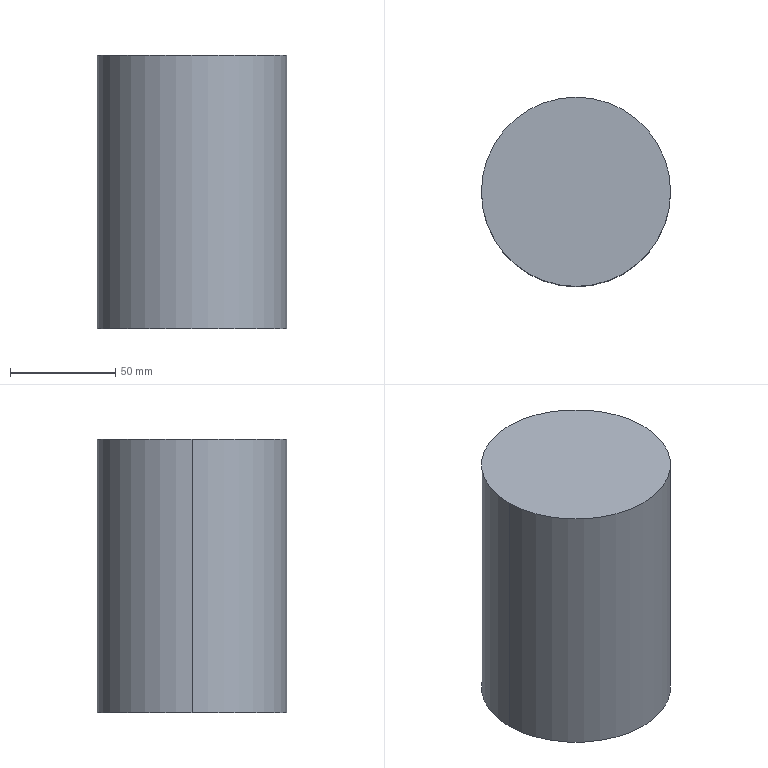Part | Creo | 1 solid | 11 faces | box 90 x 90 x 130 mm | volume 824415 mm3 | cylinder 6 | plane 3 | cone 2 | commonest cylinder face diameters 10.5 x2 12 x2 90 x2
STEP:
#1=CARTESIAN_POINT('',(-40.,-90.005,-201.));
#2=VERTEX_POINT('',#1);
#3=CARTESIAN_POINT('',(50.,-90.005,-201.));
#4=VERTEX_POINT('',#3);
#5=CARTESIAN_POINT('',(5.,-90.005,-201.));
#6=DIRECTION('',(0.,0.,1.));
#7=DIRECTION('',(-1.,0.,0.));
#8=AXIS2_PLACEMENT_3D('',#5,#6,#7);
#9=CIRCLE('',#8,45.);
#10=EDGE_CURVE('',#2,#4,#9,.T.);
#11=ORIENTED_EDGE('',*,*,#10,.F.);
#12=CARTESIAN_POINT('',(5.,-90.005,-201.));
#13=DIRECTION('',(0.,0.,1.));
#14=DIRECTION('',(1.,0.,0.));
#15=AXIS2_PLACEMENT_3D('',#12,#13,#14);
#16=CIRCLE('',#15,45.);
#17=EDGE_CURVE('',#4,#2,#16,.T.);
#18=ORIENTED_EDGE('',*,*,#17,.F.);
#19=EDGE_LOOP('',(#11,#18));
#20=FACE_OUTER_BOUND('',#19,.F.);
#21=CARTESIAN_POINT('',(5.,-58.005,-201.));
#22=DIRECTION('',(0.,0.,-1.));
#23=DIRECTION('',(0.,1.,0.));
#24=AXIS2_PLACEMENT_3D('',#21,#22,#23);
#25=PLANE('',#24);
#26=ADVANCED_FACE('',(#20),#25,.F.);
#27=ORIENTED_EDGE('',*,*,#10,.T.);
#28=CARTESIAN_POINT('',(50.,-90.005,-331.));
#29=VERTEX_POINT('',#28);
#30=CARTESIAN_POINT('',(50.,-90.005,-331.));
#31=DIRECTION('',(0.,0.,1.));
#32=VECTOR('',#31,130.);
#33=LINE('',#30,#32);
#34=EDGE_CURVE('',#29,#4,#33,.T.);
#35=ORIENTED_EDGE('',*,*,#34,.F.);
#36=CARTESIAN_POINT('',(-40.,-90.005,-331.));
#37=VERTEX_POINT('',#36);
#38=CARTESIAN_POINT('',(5.,-90.005,-331.));
#39=DIRECTION('',(0.,0.,-1.));
#40=DIRECTION('',(1.,0.,0.));
#41=AXIS2_PLACEMENT_3D('',#38,#39,#40);
#42=CIRCLE('',#41,45.);
#43=EDGE_CURVE('',#29,#37,#42,.T.);
#44=ORIENTED_EDGE('',*,*,#43,.T.);
#45=CARTESIAN_POINT('',(-40.,-90.005,-331.));
#46=DIRECTION('',(0.,0.,1.));
#47=VECTOR('',#46,130.);
#48=LINE('',#45,#47);
#49=EDGE_CURVE('',#37,#2,#48,.T.);
#50=ORIENTED_EDGE('',*,*,#49,.T.);
#51=EDGE_LOOP('',(#27,#35,#44,#50));
#52=FACE_OUTER_BOUND('',#51,.F.);
#53=CARTESIAN_POINT('',(5.,-90.005,-401.));
#54=DIRECTION('',(0.,0.,1.));
#55=DIRECTION('',(1.,0.,0.));
#56=AXIS2_PLACEMENT_3D('',#53,#54,#55);
#57=CYLINDRICAL_SURFACE('',#56,45.);
#58=ADVANCED_FACE('',(#52),#57,.T.);
#59=ORIENTED_EDGE('',*,*,#17,.T.);
#60=ORIENTED_EDGE('',*,*,#49,.F.);
#61=CARTESIAN_POINT('',(5.,-90.005,-331.));
#62=DIRECTION('',(0.,0.,-1.));
#63=DIRECTION('',(-1.,0.,0.));
#64=AXIS2_PLACEMENT_3D('',#61,#62,#63);
#65=CIRCLE('',#64,45.);
#66=EDGE_CURVE('',#37,#29,#65,.T.);
#67=ORIENTED_EDGE('',*,*,#66,.T.);
#68=ORIENTED_EDGE('',*,*,#34,.T.);
#69=EDGE_LOOP('',(#59,#60,#67,#68));
#70=FACE_OUTER_BOUND('',#69,.F.);
#71=CARTESIAN_POINT('',(5.,-90.005,-401.));
#72=DIRECTION('',(0.,0.,1.));
#73=DIRECTION('',(1.,0.,0.));
#74=AXIS2_PLACEMENT_3D('',#71,#72,#73);
#75=CYLINDRICAL_SURFACE('',#74,45.);
#76=ADVANCED_FACE('',(#70),#75,.T.);
#77=ORIENTED_EDGE('',*,*,#43,.F.);
#78=ORIENTED_EDGE('',*,*,#66,.F.);
#79=EDGE_LOOP('',(#77,#78));
#80=FACE_OUTER_BOUND('',#79,.F.);
#81=CARTESIAN_POINT('',(11.,-90.005,-331.));
#82=VERTEX_POINT('',#81);
#83=CARTESIAN_POINT('',(-1.,-90.005,-331.));
#84=VERTEX_POINT('',#83);
#85=CARTESIAN_POINT('',(5.,-90.005,-331.));
#86=DIRECTION('',(0.,0.,1.));
#87=DIRECTION('',(1.,0.,0.));
#88=AXIS2_PLACEMENT_3D('',#85,#86,#87);
#89=CIRCLE('',#88,6.);
#90=EDGE_CURVE('',#82,#84,#89,.T.);
#91=ORIENTED_EDGE('',*,*,#90,.F.);
#92=CARTESIAN_POINT('',(5.,-90.005,-331.));
#93=DIRECTION('',(0.,0.,1.));
#94=DIRECTION('',(-1.,0.,0.));
#95=AXIS2_PLACEMENT_3D('',#92,#93,#94);
#96=CIRCLE('',#95,6.);
#97=EDGE_CURVE('',#84,#82,#96,.T.);
#98=ORIENTED_EDGE('',*,*,#97,.F.);
#99=EDGE_LOOP('',(#91,#98));
#100=FACE_BOUND('',#99,.F.);
#101=CARTESIAN_POINT('',(15.,-0.004699,-331.));
#102=DIRECTION('',(0.,0.,1.));
#103=DIRECTION('',(0.,1.,0.));
#104=AXIS2_PLACEMENT_3D('',#101,#102,#103);
#105=PLANE('',#104);
#106=ADVANCED_FACE('',(#80,#100),#105,.F.);
#107=ORIENTED_EDGE('',*,*,#90,.T.);
#108=CARTESIAN_POINT('',(-1.,-90.005,-311.));
#109=VERTEX_POINT('',#108);
#110=CARTESIAN_POINT('',(-1.,-90.005,-331.));
#111=DIRECTION('',(0.,0.,1.));
#112=VECTOR('',#111,20.);
#113=LINE('',#110,#112);
#114=EDGE_CURVE('',#84,#109,#113,.T.);
#115=ORIENTED_EDGE('',*,*,#114,.T.);
#116=CARTESIAN_POINT('',(11.,-90.005,-311.));
#117=VERTEX_POINT('',#116);
#118=CARTESIAN_POINT('',(5.,-90.005,-311.));
#119=DIRECTION('',(0.,0.,-1.));
#120=DIRECTION('',(-1.,0.,0.));
#121=AXIS2_PLACEMENT_3D('',#118,#119,#120);
#122=CIRCLE('',#121,6.);
#123=EDGE_CURVE('',#109,#117,#122,.T.);
#124=ORIENTED_EDGE('',*,*,#123,.T.);
#125=CARTESIAN_POINT('',(11.,-90.005,-331.));
#126=DIRECTION('',(0.,0.,1.));
#127=VECTOR('',#126,20.);
#128=LINE('',#125,#127);
#129=EDGE_CURVE('',#82,#117,#128,.T.);
#130=ORIENTED_EDGE('',*,*,#129,.F.);
#131=EDGE_LOOP('',(#107,#115,#124,#130));
#132=FACE_OUTER_BOUND('',#131,.F.);
#133=CARTESIAN_POINT('',(5.,-90.005,-366.));
#134=DIRECTION('',(0.,0.,1.));
#135=DIRECTION('',(1.,0.,0.));
#136=AXIS2_PLACEMENT_3D('',#133,#134,#135);
#137=CYLINDRICAL_SURFACE('',#136,6.);
#138=ADVANCED_FACE('',(#132),#137,.F.);
#139=ORIENTED_EDGE('',*,*,#97,.T.);
#140=ORIENTED_EDGE('',*,*,#129,.T.);
#141=CARTESIAN_POINT('',(5.,-90.005,-311.));
#142=DIRECTION('',(0.,0.,-1.));
#143=DIRECTION('',(1.,0.,0.));
#144=AXIS2_PLACEMENT_3D('',#141,#142,#143);
#145=CIRCLE('',#144,6.);
#146=EDGE_CURVE('',#117,#109,#145,.T.);
#147=ORIENTED_EDGE('',*,*,#146,.T.);
#148=ORIENTED_EDGE('',*,*,#114,.F.);
#149=EDGE_LOOP('',(#139,#140,#147,#148));
#150=FACE_OUTER_BOUND('',#149,.F.);
#151=CARTESIAN_POINT('',(5.,-90.005,-366.));
#152=DIRECTION('',(0.,0.,1.));
#153=DIRECTION('',(1.,0.,0.));
#154=AXIS2_PLACEMENT_3D('',#151,#152,#153);
#155=CYLINDRICAL_SURFACE('',#154,6.);
#156=ADVANCED_FACE('',(#150),#155,.F.);
#157=ORIENTED_EDGE('',*,*,#146,.F.);
#158=ORIENTED_EDGE('',*,*,#123,.F.);
#159=EDGE_LOOP('',(#157,#158));
#160=FACE_OUTER_BOUND('',#159,.F.);
#161=CARTESIAN_POINT('',(10.25,-90.005,-311.));
#162=VERTEX_POINT('',#161);
#163=CARTESIAN_POINT('',(-0.25,-90.005,-311.));
#164=VERTEX_POINT('',#163);
#165=CARTESIAN_POINT('',(5.,-90.005,-311.));
#166=DIRECTION('',(0.,0.,1.));
#167=DIRECTION('',(1.,0.,0.));
#168=AXIS2_PLACEMENT_3D('',#165,#166,#167);
#169=CIRCLE('',#168,5.25);
#170=EDGE_CURVE('',#162,#164,#169,.T.);
#171=ORIENTED_EDGE('',*,*,#170,.F.);
#172=CARTESIAN_POINT('',(5.,-90.005,-311.));
#173=DIRECTION('',(0.,0.,1.));
#174=DIRECTION('',(-1.,0.,0.));
#175=AXIS2_PLACEMENT_3D('',#172,#173,#174);
#176=CIRCLE('',#175,5.25);
#177=EDGE_CURVE('',#164,#162,#176,.T.);
#178=ORIENTED_EDGE('',*,*,#177,.F.);
#179=EDGE_LOOP('',(#171,#178));
#180=FACE_BOUND('',#179,.F.);
#181=CARTESIAN_POINT('',(5.,-90.005,-311.));
#182=DIRECTION('',(0.,0.,1.));
#183=DIRECTION('',(1.,0.,0.));
#184=AXIS2_PLACEMENT_3D('',#181,#182,#183);
#185=PLANE('',#184);
#186=ADVANCED_FACE('',(#160,#180),#185,.F.);
#187=ORIENTED_EDGE('',*,*,#170,.T.);
#188=CARTESIAN_POINT('',(-0.25,-90.005,-308.));
#189=VERTEX_POINT('',#188);
#190=CARTESIAN_POINT('',(-0.25,-90.005,-311.));
#191=DIRECTION('',(0.,0.,1.));
#192=VECTOR('',#191,3.);
#193=LINE('',#190,#192);
#194=EDGE_CURVE('',#164,#189,#193,.T.);
#195=ORIENTED_EDGE('',*,*,#194,.T.);
#196=CARTESIAN_POINT('',(10.25,-90.005,-308.));
#197=VERTEX_POINT('',#196);
#198=CARTESIAN_POINT('',(5.,-90.005,-308.));
#199=DIRECTION('',(0.,0.,-1.));
#200=DIRECTION('',(-1.,0.,0.));
#201=AXIS2_PLACEMENT_3D('',#198,#199,#200);
#202=CIRCLE('',#201,5.25);
#203=EDGE_CURVE('',#189,#197,#202,.T.);
#204=ORIENTED_EDGE('',*,*,#203,.T.);
#205=CARTESIAN_POINT('',(10.25,-90.005,-311.));
#206=DIRECTION('',(0.,0.,1.));
#207=VECTOR('',#206,3.);
#208=LINE('',#205,#207);
#209=EDGE_CURVE('',#162,#197,#208,.T.);
#210=ORIENTED_EDGE('',*,*,#209,.F.);
#211=EDGE_LOOP('',(#187,#195,#204,#210));
#212=FACE_OUTER_BOUND('',#211,.F.);
#213=CARTESIAN_POINT('',(5.,-90.005,-366.));
#214=DIRECTION('',(0.,0.,1.));
#215=DIRECTION('',(1.,0.,0.));
#216=AXIS2_PLACEMENT_3D('',#213,#214,#215);
#217=CYLINDRICAL_SURFACE('',#216,5.25);
#218=ADVANCED_FACE('',(#212),#217,.F.);
#219=ORIENTED_EDGE('',*,*,#177,.T.);
#220=ORIENTED_EDGE('',*,*,#209,.T.);
#221=CARTESIAN_POINT('',(5.,-90.005,-308.));
#222=DIRECTION('',(0.,0.,-1.));
#223=DIRECTION('',(1.,0.,0.));
#224=AXIS2_PLACEMENT_3D('',#221,#222,#223);
#225=CIRCLE('',#224,5.25);
#226=EDGE_CURVE('',#197,#189,#225,.T.);
#227=ORIENTED_EDGE('',*,*,#226,.T.);
#228=ORIENTED_EDGE('',*,*,#194,.F.);
#229=EDGE_LOOP('',(#219,#220,#227,#228));
#230=FACE_OUTER_BOUND('',#229,.F.);
#231=CARTESIAN_POINT('',(5.,-90.005,-366.));
#232=DIRECTION('',(0.,0.,1.));
#233=DIRECTION('',(1.,0.,0.));
#234=AXIS2_PLACEMENT_3D('',#231,#232,#233);
#235=CYLINDRICAL_SURFACE('',#234,5.25);
#236=ADVANCED_FACE('',(#230),#235,.F.);
#237=ORIENTED_EDGE('',*,*,#226,.F.);
#238=CARTESIAN_POINT('',(5.,-90.005,-304.969));
#239=VERTEX_POINT('',#238);
#240=CARTESIAN_POINT('',(5.,-90.005,-304.969));
#241=DIRECTION('',(0.866,0.,-0.5));
#242=VECTOR('',#241,6.062);
#243=LINE('',#240,#242);
#244=EDGE_CURVE('',#239,#197,#243,.T.);
#245=ORIENTED_EDGE('',*,*,#244,.F.);
#246=CARTESIAN_POINT('',(5.,-90.005,-304.969));
#247=DIRECTION('',(-0.866,0.,-0.5));
#248=VECTOR('',#247,6.062);
#249=LINE('',#246,#248);
#250=EDGE_CURVE('',#239,#189,#249,.T.);
#251=ORIENTED_EDGE('',*,*,#250,.T.);
#252=EDGE_LOOP('',(#237,#245,#251));
#253=FACE_OUTER_BOUND('',#252,.F.);
#254=CARTESIAN_POINT('',(5.,-90.005,-306.539));
#255=DIRECTION('',(0.,0.,-1.));
#256=DIRECTION('',(-1.,0.,0.));
#257=AXIS2_PLACEMENT_3D('',#254,#255,#256);
#258=CONICAL_SURFACE('',#257,2.72,60.);
#259=ADVANCED_FACE('',(#253),#258,.F.);
#260=ORIENTED_EDGE('',*,*,#203,.F.);
#261=ORIENTED_EDGE('',*,*,#250,.F.);
#262=ORIENTED_EDGE('',*,*,#244,.T.);
#263=EDGE_LOOP('',(#260,#261,#262));
#264=FACE_OUTER_BOUND('',#263,.F.);
#265=CARTESIAN_POINT('',(5.,-90.005,-306.539));
#266=DIRECTION('',(0.,0.,-1.));
#267=DIRECTION('',(-1.,0.,0.));
#268=AXIS2_PLACEMENT_3D('',#265,#266,#267);
#269=CONICAL_SURFACE('',#268,2.72,60.);
#270=ADVANCED_FACE('',(#264),#269,.F.);
#271=CLOSED_SHELL('',(#26,#58,#76,#106,#138,#156,#186,#218,#236,#259,#270));
#272=MANIFOLD_SOLID_BREP('',#271);
#273=(LENGTH_UNIT()NAMED_UNIT(*)SI_UNIT(.MILLI.,.METRE.));
#274=UNCERTAINTY_MEASURE_WITH_UNIT(LENGTH_MEASURE(0.0182),#273,'','');
#275=(NAMED_UNIT(*)PLANE_ANGLE_UNIT()SI_UNIT($,.RADIAN.));
#276=PLANE_ANGLE_MEASURE_WITH_UNIT(PLANE_ANGLE_MEASURE(0.01745),#275);
#277=(CONVERSION_BASED_UNIT('DEGREE',#276)NAMED_UNIT(*)PLANE_ANGLE_UNIT());
#278=(NAMED_UNIT(*)SI_UNIT($,.STERADIAN.)SOLID_ANGLE_UNIT());
#279=(GEOMETRIC_REPRESENTATION_CONTEXT(3)GLOBAL_UNCERTAINTY_ASSIGNED_CONTEXT((#274))GLOBAL_UNIT_ASSIGNED_CONTEXT((#273,#277,#278))REPRESENTATION_CONTEXT('',''));
#280=ADVANCED_BREP_SHAPE_REPRESENTATION('',(#272),#279);